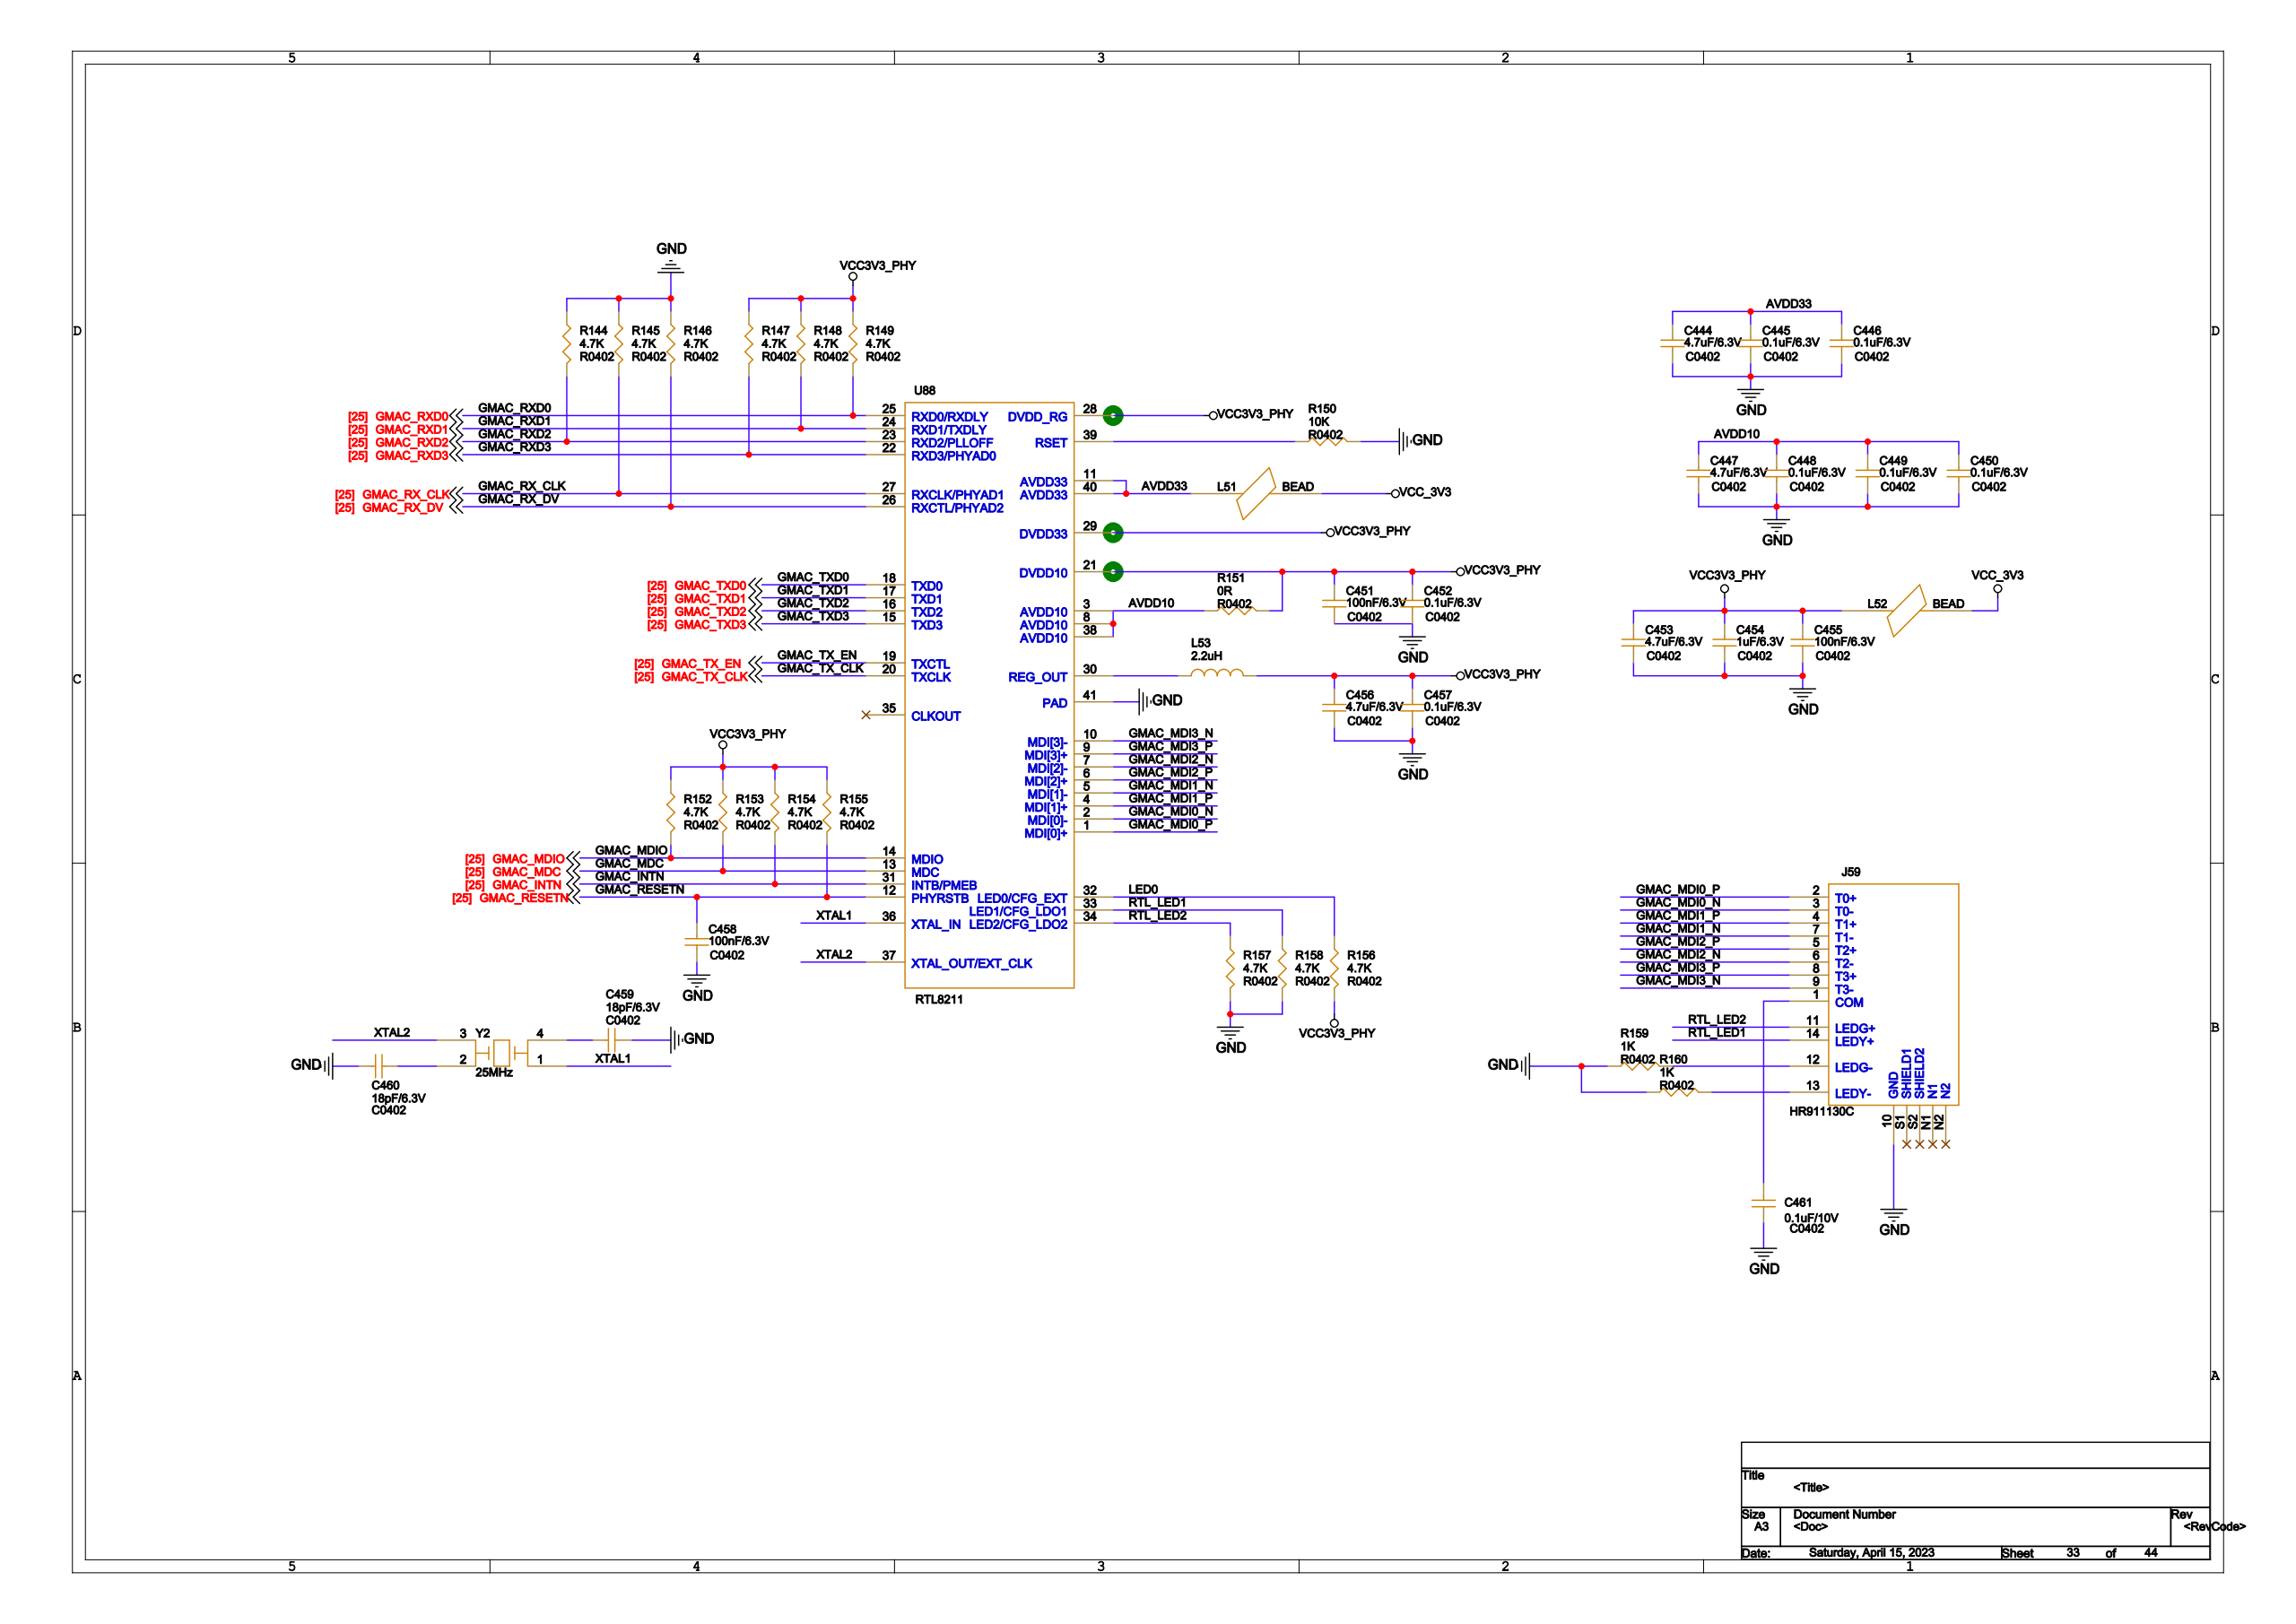Circuit board | Cadence Allegro | 1034 parts | 912 nets | one sheet of the schematic
Parts on this sheet (reference | value | footprint):
C444 | 4.7uF/6.3V | C0402
C445 | 0.1uF/6.3V | C0402
C446 | 0.1uF/6.3V | C0402
C447 | 4.7uF/6.3V | C0402
C448 | 0.1uF/6.3V | C0402
C449 | 0.1uF/6.3V | C0402
C450 | 0.1uF/6.3V | C0402
C451 | 100nF/6.3V | C0402
C452 | 0.1uF/6.3V | C0402
C453 | 4.7uF/6.3V | C0402
C454 | 1uF/6.3V | C0402
C455 | 100nF/6.3V | C0402
C456 | 4.7uF/6.3V | C0402
C457 | 0.1uF/6.3V | C0402
C458 | 100nF/6.3V | C0402
C459 | 18pF/6.3V | C0402
C460 | 18pF/6.3V | C0402
C461 | 0.1uF/10V | C0402
J59 | HR911130C | HR911130C
L51 | BEAD | PZ2012
L52 | BEAD | PZ2012
L53 | 2.2uH | L252010
R144 | 4.7k | R0402
R145 | 4.7k | R0402
R146 | 4.7k | R0402
R147 | 4.7k | R0402
R148 | 4.7k | R0402
R149 | 4.7k | R0402
R150 | 10k | R0402
R151 | 0R | R0402
R152 | 4.7k | R0402
R153 | 4.7k | R0402
R154 | 4.7k | R0402
R155 | 4.7k | R0402
R156 | 4.7k | R0402
R157 | 4.7k | R0402
R158 | 4.7k | R0402
R159 | 1K | R0402
R160 | 1K | R0402
U88 | RTL8211 | QFN_8211
Y2 | 25MHz | 3225
Nets of these parts (net: part-pin ...):
GND: C444-2 C445-2 C446-2 C447-2 C448-2 C449-2 C450-2 C451-2 C452-2 C453-2 C454-2 C455-2 C456-2 C457-2 C458-2 C459-2 C460-2 C461-1 J59-10 R144-1 R145-1 R146-1 R150-2 R157-2 R158-2 R159-1 R160-1 U88-41
VCC_3V3: L51-2 L52-2
AVDD33: C444-1 C445-1 C446-1 L51-1 U88-11 U88-40
AVDD10: C447-1 C448-1 C449-1 C450-1 R151-1 U88-3 U88-8 U88-38
VCC3V3_PHY: C451-1 C452-1 C453-1 C454-1 C455-1 C456-1 C457-1 L52-1 L53-2 R147-1 R148-1 R149-1 R151-2 R152-1 R153-1 R154-1 R155-1 R156-2 U88-21 U88-28 U88-29
N14235723: C459-1 Y2-4
N14235757: C460-1 Y2-2
N14764250: C461-2 J59-1
N14237084: J59-12 R159-2
N14763174: J59-13 R160-2
RTL_LED2: J59-11 R157-1 U88-34
RTL_LED1: J59-14 R158-1 U88-33
GMAC_MDI0_P: J59-2 U88-1
GMAC_MDI0_N: J59-3 U88-2
GMAC_MDI1_P: J59-4 U88-4
GMAC_MDI1_N: J59-7 U88-5
GMAC_MDI2_P: J59-5 U88-6
GMAC_MDI2_N: J59-6 U88-7
GMAC_MDI3_P: J59-8 U88-9
GMAC_MDI3_N: J59-9 U88-10
GMAC_RESETN: C458-1 R155-2 U88-12
N14235073: L53-1 U88-30
GMAC_RXD1: R148-2 U88-24
GMAC_RXD0: R149-2 U88-25
GMAC_RXD2: R144-2 U88-23
GMAC_RX_CLK: R145-2 U88-27
GMAC_RX_DV: R146-2 U88-26
GMAC_RXD3: R147-2 U88-22
GMAC_MDIO: R152-2 U88-14
GMAC_MDC: R153-2 U88-13
GMAC_INTN: R154-2 U88-31
LED0: R156-1 U88-32
N14234437: R150-1 U88-39
GMAC_TX_CLK: U88-20
GMAC_TXD1: U88-17
GMAC_TXD0: U88-18
GMAC_TXD3: U88-15
GMAC_TXD2: U88-16
GMAC_TX_EN: U88-19
XTAL1: Y2-1 U88-36
XTAL2: Y2-3 U88-37